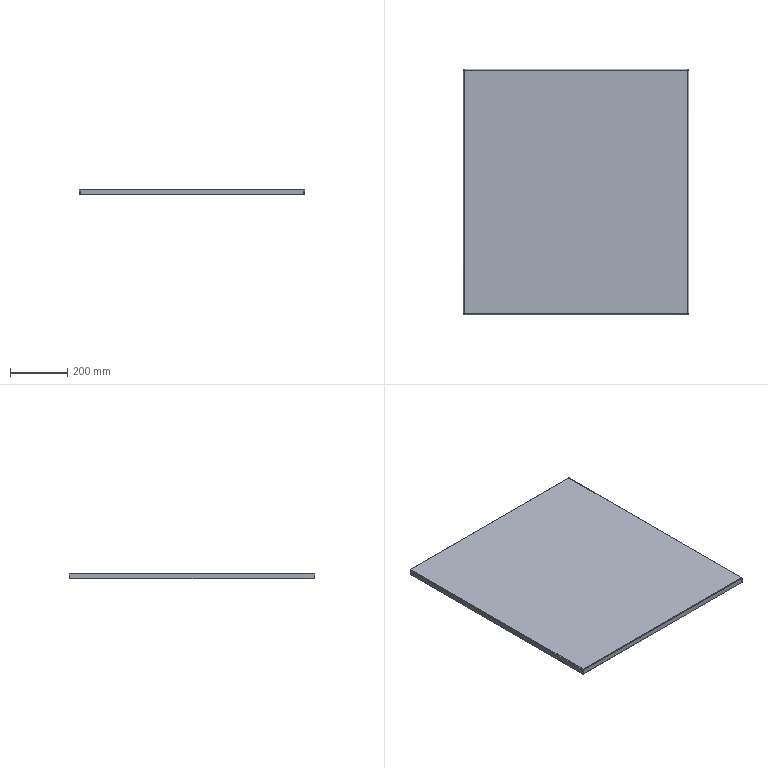Part | STEP file | 001-001-Machine frame bottom end plate | 1 solid | 38 faces | box 788 x 858 x 20 mm | volume 1465006 mm3 | plane 22 | spline 8 | cylinder 8 | commonest cylinder face diameters 1.473 x4 5.473 x4